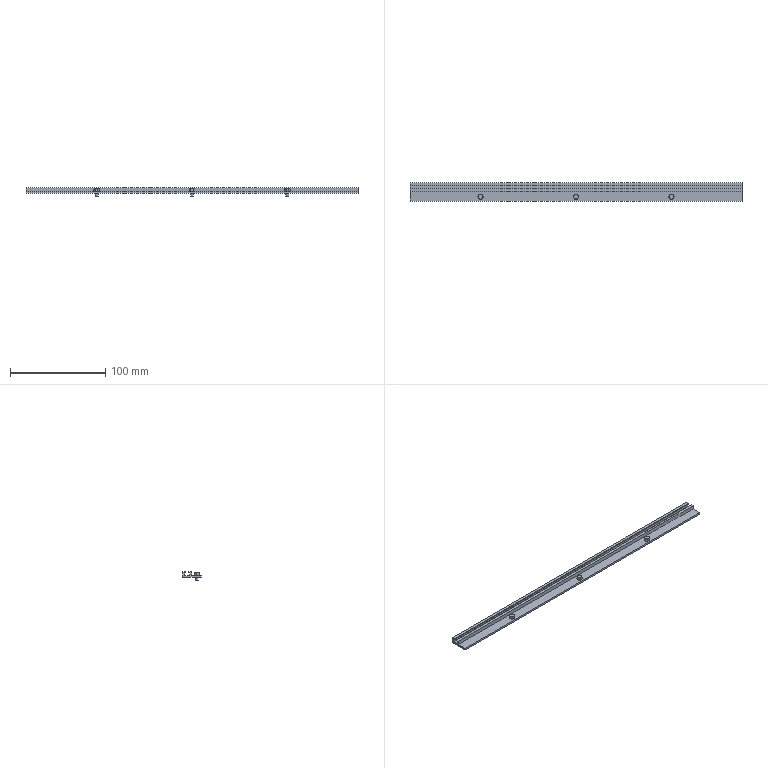Part | STEP file | Guide wheel mechanism revised.sldasm-Part-420 | 1 solid | 115 faces | box 348 x 19 x 9 mm | volume 19396 mm3 | cone 48 | plane 40 | cylinder 27 | commonest cylinder face diameters 5.765 x21 3 x6